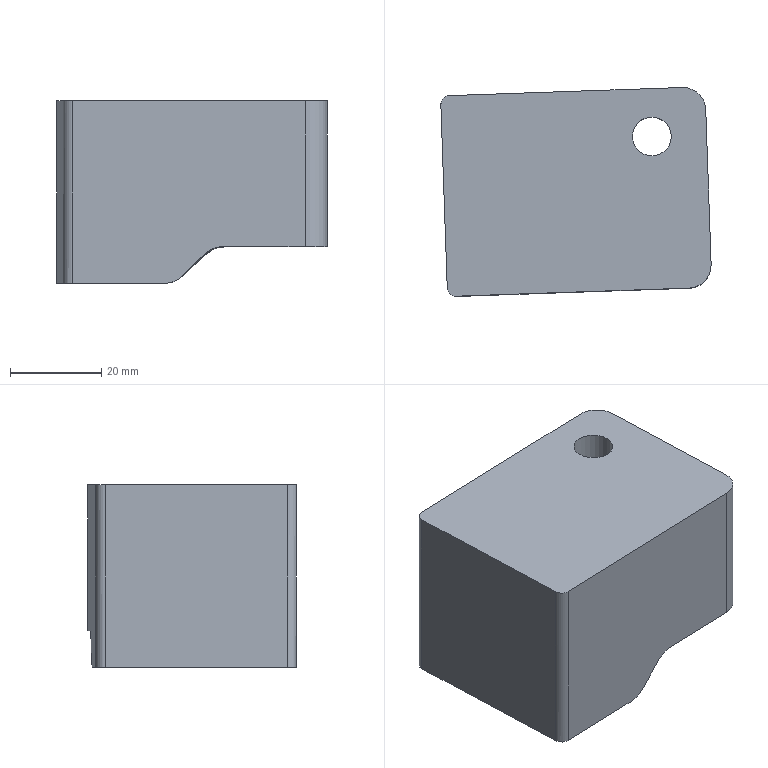Part | NX | features PS-16 2 | 1 solid | 16 faces | box 59.26 x 45.757 x 40 mm | volume 88557 mm3 | plane 8 | cylinder 6 | spline 2 | commonest cylinder face diameters 4 x2 10 x2 8.506 x1 14.5 x1
STEP:
#1=CARTESIAN_POINT('',(2975.173,-776.36,868.716));
#2=VERTEX_POINT('',#1);
#3=CARTESIAN_POINT('',(2958.185,-776.954,868.716));
#4=VERTEX_POINT('',#3);
#5=CARTESIAN_POINT('',(2937.196,-777.686,868.716));
#6=DIRECTION('',(-0.9994,-0.0349,0.));
#7=VECTOR('',#6,1000.);
#8=LINE('',#5,#7);
#9=EDGE_CURVE('',#2,#4,#8,.T.);
#10=ORIENTED_EDGE('',*,*,#9,.F.);
#11=CARTESIAN_POINT('',(2980.345,-781.183,868.716));
#12=VERTEX_POINT('',#11);
#13=CARTESIAN_POINT('',(2975.348,-781.357,868.716));
#14=DIRECTION('',(0.,0.,1.));
#15=DIRECTION('',(-1.,0.,0.));
#16=AXIS2_PLACEMENT_3D('',#13,#14,#15);
#17=CIRCLE('',#16,5.);
#18=EDGE_CURVE('',#12,#2,#17,.T.);
#19=ORIENTED_EDGE('',*,*,#18,.F.);
#20=CARTESIAN_POINT('',(2981.531,-815.162,868.716));
#21=VERTEX_POINT('',#20);
#22=CARTESIAN_POINT('',(2981.283,-808.048,868.716));
#23=DIRECTION('',(-0.0349,0.9994,0.));
#24=VECTOR('',#23,1000.);
#25=LINE('',#22,#24);
#26=EDGE_CURVE('',#21,#12,#25,.T.);
#27=ORIENTED_EDGE('',*,*,#26,.F.);
#28=CARTESIAN_POINT('',(2976.709,-820.334,868.716));
#29=VERTEX_POINT('',#28);
#30=CARTESIAN_POINT('',(2976.534,-815.337,868.716));
#31=DIRECTION('',(0.,0.,1.));
#32=DIRECTION('',(-1.,0.,0.));
#33=AXIS2_PLACEMENT_3D('',#30,#31,#32);
#34=CIRCLE('',#33,5.);
#35=EDGE_CURVE('',#29,#21,#34,.T.);
#36=ORIENTED_EDGE('',*,*,#35,.F.);
#37=CARTESIAN_POINT('',(2959.023,-820.951,868.716));
#38=VERTEX_POINT('',#37);
#39=CARTESIAN_POINT('',(2967.654,-820.65,868.716));
#40=DIRECTION('',(0.9994,0.0349,0.));
#41=VECTOR('',#40,1000.);
#42=LINE('',#39,#41);
#43=EDGE_CURVE('',#38,#29,#42,.T.);
#44=ORIENTED_EDGE('',*,*,#43,.F.);
#45=CARTESIAN_POINT('',(2958.185,-796.966,868.716));
#46=VERTEX_POINT('',#45);
#47=CARTESIAN_POINT('',(2958.011,-791.963,868.716));
#48=DIRECTION('',(-0.0349,0.9994,0.));
#49=VECTOR('',#48,1000.);
#50=LINE('',#47,#49);
#51=EDGE_CURVE('',#46,#38,#50,.F.);
#52=ORIENTED_EDGE('',*,*,#51,.F.);
#53=CARTESIAN_POINT('',(2958.185,-776.954,868.716));
#54=CARTESIAN_POINT('',(2958.185,-777.787,868.716));
#55=CARTESIAN_POINT('',(2958.185,-779.456,868.716));
#56=CARTESIAN_POINT('',(2958.185,-781.955,868.716));
#57=CARTESIAN_POINT('',(2958.185,-784.047,868.716));
#58=CARTESIAN_POINT('',(2958.185,-785.492,868.716));
#59=CARTESIAN_POINT('',(2958.185,-786.349,868.716));
#60=CARTESIAN_POINT('',(2958.185,-786.904,868.716));
#61=CARTESIAN_POINT('',(2958.185,-787.793,868.716));
#62=CARTESIAN_POINT('',(2958.185,-788.774,868.716));
#63=CARTESIAN_POINT('',(2958.185,-789.914,868.716));
#64=CARTESIAN_POINT('',(2958.185,-791.068,868.716));
#65=CARTESIAN_POINT('',(2958.185,-791.963,868.716));
#66=CARTESIAN_POINT('',(2958.185,-792.857,868.716));
#67=CARTESIAN_POINT('',(2958.185,-794.4,868.716));
#68=CARTESIAN_POINT('',(2958.185,-795.854,868.716));
#69=CARTESIAN_POINT('',(2958.185,-796.966,868.716));
#70=B_SPLINE_CURVE_WITH_KNOTS('',3,(#53,#54,#55,#56,#57,#58,#59,#60,#61,#62,#63,#64,#65,#66,#67,#68,#69),.UNSPECIFIED.,.F.,.F.,(4,1,1,1,1,1,1,1,1,1,1,1,1,1,4),(0.,0.125,0.25,0.375,0.4375,0.4688,0.5,0.5312,0.5625,0.625,0.6875,0.75,0.8125,0.875,1.),.UNSPECIFIED.);
#71=EDGE_CURVE('',#46,#4,#70,.F.);
#72=ORIENTED_EDGE('',*,*,#71,.T.);
#73=EDGE_LOOP('',(#10,#19,#27,#36,#44,#52,#72));
#74=FACE_BOUND('',#73,.T.);
#75=CARTESIAN_POINT('',(2975.794,-787.098,868.716));
#76=VERTEX_POINT('',#75);
#77=CARTESIAN_POINT('',(2968.544,-787.098,868.716));
#78=DIRECTION('',(0.,0.,-1.));
#79=DIRECTION('',(1.,0.,0.));
#80=AXIS2_PLACEMENT_3D('',#77,#78,#79);
#81=CIRCLE('',#80,7.25);
#82=EDGE_CURVE('',#76,#76,#81,.T.);
#83=ORIENTED_EDGE('',*,*,#82,.F.);
#84=EDGE_LOOP('',(#83));
#85=FACE_BOUND('',#84,.T.);
#86=CARTESIAN_POINT('',(2967.231,-808.539,868.716));
#87=DIRECTION('',(0.,0.,-1.));
#88=DIRECTION('',(0.0349,-0.9994,0.));
#89=AXIS2_PLACEMENT_3D('',#86,#87,#88);
#90=PLANE('',#89);
#91=ADVANCED_FACE('',(#74,#85),#90,.T.);
#92=CARTESIAN_POINT('',(2923.671,-820.184,900.716));
#93=VERTEX_POINT('',#92);
#94=CARTESIAN_POINT('',(2922.275,-780.209,900.716));
#95=VERTEX_POINT('',#94);
#96=CARTESIAN_POINT('',(2924.945,-856.656,900.716));
#97=DIRECTION('',(-0.0349,0.9994,0.));
#98=VECTOR('',#97,1000.);
#99=LINE('',#96,#98);
#100=EDGE_CURVE('',#93,#95,#99,.T.);
#101=ORIENTED_EDGE('',*,*,#100,.T.);
#102=CARTESIAN_POINT('',(2922.275,-780.209,860.716));
#103=VERTEX_POINT('',#102);
#104=CARTESIAN_POINT('',(2922.275,-780.209,862.716));
#105=DIRECTION('',(0.,0.,-1.));
#106=VECTOR('',#105,1000.);
#107=LINE('',#104,#106);
#108=EDGE_CURVE('',#103,#95,#107,.F.);
#109=ORIENTED_EDGE('',*,*,#108,.F.);
#110=CARTESIAN_POINT('',(2923.671,-820.184,860.716));
#111=VERTEX_POINT('',#110);
#112=CARTESIAN_POINT('',(2923.671,-820.184,860.716));
#113=CARTESIAN_POINT('',(2923.206,-806.859,860.716));
#114=CARTESIAN_POINT('',(2922.741,-793.534,860.716));
#115=CARTESIAN_POINT('',(2922.275,-780.209,860.716));
#116=B_SPLINE_CURVE_WITH_KNOTS('',3,(#112,#113,#114,#115),.UNSPECIFIED.,.F.,.F.,(4,4),(0.,0.04),.UNSPECIFIED.);
#117=EDGE_CURVE('',#111,#103,#116,.T.);
#118=ORIENTED_EDGE('',*,*,#117,.F.);
#119=CARTESIAN_POINT('',(2923.671,-820.184,862.716));
#120=DIRECTION('',(0.,0.,-1.));
#121=VECTOR('',#120,1000.);
#122=LINE('',#119,#121);
#123=EDGE_CURVE('',#93,#111,#122,.T.);
#124=ORIENTED_EDGE('',*,*,#123,.F.);
#125=EDGE_LOOP('',(#101,#109,#118,#124));
#126=FACE_BOUND('',#125,.T.);
#127=CARTESIAN_POINT('',(2923.132,-804.735,862.716));
#128=DIRECTION('',(0.9994,0.0349,0.));
#129=DIRECTION('',(0.0349,-0.9994,0.));
#130=AXIS2_PLACEMENT_3D('',#127,#128,#129);
#131=PLANE('',#130);
#132=ADVANCED_FACE('',(#126),#131,.F.);
#133=CARTESIAN_POINT('',(2981.531,-815.162,900.716));
#134=VERTEX_POINT('',#133);
#135=CARTESIAN_POINT('',(2981.531,-815.162,862.716));
#136=DIRECTION('',(0.,0.,1.));
#137=VECTOR('',#136,1000.);
#138=LINE('',#135,#137);
#139=EDGE_CURVE('',#21,#134,#138,.T.);
#140=ORIENTED_EDGE('',*,*,#139,.F.);
#141=ORIENTED_EDGE('',*,*,#26,.T.);
#142=CARTESIAN_POINT('',(2980.345,-781.183,900.716));
#143=VERTEX_POINT('',#142);
#144=CARTESIAN_POINT('',(2980.345,-781.183,935.716));
#145=DIRECTION('',(0.,0.,1.));
#146=VECTOR('',#145,1000.);
#147=LINE('',#144,#146);
#148=EDGE_CURVE('',#143,#12,#147,.F.);
#149=ORIENTED_EDGE('',*,*,#148,.F.);
#150=CARTESIAN_POINT('',(2982.909,-854.632,900.716));
#151=DIRECTION('',(-0.0349,0.9994,0.));
#152=VECTOR('',#151,1000.);
#153=LINE('',#150,#152);
#154=EDGE_CURVE('',#134,#143,#153,.T.);
#155=ORIENTED_EDGE('',*,*,#154,.F.);
#156=EDGE_LOOP('',(#140,#141,#149,#155));
#157=FACE_BOUND('',#156,.T.);
#158=CARTESIAN_POINT('',(2981.096,-802.711,862.716));
#159=DIRECTION('',(0.9994,0.0349,0.));
#160=DIRECTION('',(0.0349,-0.9994,0.));
#161=AXIS2_PLACEMENT_3D('',#158,#159,#160);
#162=PLANE('',#161);
#163=ADVANCED_FACE('',(#157),#162,.T.);
#164=CARTESIAN_POINT('',(2975.173,-776.36,900.716));
#165=VERTEX_POINT('',#164);
#166=CARTESIAN_POINT('',(2924.204,-778.14,900.716));
#167=VERTEX_POINT('',#166);
#168=CARTESIAN_POINT('',(2937.196,-777.686,900.716));
#169=DIRECTION('',(-0.9994,-0.0349,0.));
#170=VECTOR('',#169,1000.);
#171=LINE('',#168,#170);
#172=EDGE_CURVE('',#165,#167,#171,.T.);
#173=ORIENTED_EDGE('',*,*,#172,.F.);
#174=CARTESIAN_POINT('',(2975.173,-776.36,935.716));
#175=DIRECTION('',(0.,0.,1.));
#176=VECTOR('',#175,1000.);
#177=LINE('',#174,#176);
#178=EDGE_CURVE('',#2,#165,#177,.T.);
#179=ORIENTED_EDGE('',*,*,#178,.F.);
#180=ORIENTED_EDGE('',*,*,#9,.T.);
#181=CARTESIAN_POINT('',(2946.238,-777.371,860.716));
#182=VERTEX_POINT('',#181);
#183=CARTESIAN_POINT('',(2946.238,-777.371,860.716));
#184=CARTESIAN_POINT('',(2946.843,-777.35,860.716));
#185=CARTESIAN_POINT('',(2948.076,-777.307,860.995));
#186=CARTESIAN_POINT('',(2950.148,-777.234,862.36));
#187=CARTESIAN_POINT('',(2952.239,-777.161,864.66));
#188=CARTESIAN_POINT('',(2954.666,-777.076,867.458));
#189=CARTESIAN_POINT('',(2956.946,-776.997,868.716));
#190=CARTESIAN_POINT('',(2958.185,-776.954,868.716));
#191=B_SPLINE_CURVE_WITH_KNOTS('',3,(#183,#184,#185,#186,#187,#188,#189,#190),.UNSPECIFIED.,.F.,.F.,(4,1,1,1,1,4),(0.008073,0.009904,0.01173,0.0154,0.01906,0.02272),.UNSPECIFIED.);
#192=EDGE_CURVE('',#4,#182,#191,.F.);
#193=ORIENTED_EDGE('',*,*,#192,.T.);
#194=CARTESIAN_POINT('',(2924.204,-778.14,860.716));
#195=VERTEX_POINT('',#194);
#196=CARTESIAN_POINT('',(2924.204,-778.14,860.716));
#197=CARTESIAN_POINT('',(2931.549,-777.884,860.716));
#198=CARTESIAN_POINT('',(2938.894,-777.627,860.716));
#199=CARTESIAN_POINT('',(2946.238,-777.371,860.716));
#200=B_SPLINE_CURVE_WITH_KNOTS('',3,(#196,#197,#198,#199),.UNSPECIFIED.,.F.,.F.,(4,4),(0.,0.02205),.UNSPECIFIED.);
#201=EDGE_CURVE('',#195,#182,#200,.T.);
#202=ORIENTED_EDGE('',*,*,#201,.F.);
#203=CARTESIAN_POINT('',(2924.204,-778.14,935.716));
#204=DIRECTION('',(0.,0.,-1.));
#205=VECTOR('',#204,1000.);
#206=LINE('',#203,#205);
#207=EDGE_CURVE('',#167,#195,#206,.T.);
#208=ORIENTED_EDGE('',*,*,#207,.F.);
#209=EDGE_LOOP('',(#173,#179,#180,#193,#202,#208));
#210=FACE_BOUND('',#209,.T.);
#211=CARTESIAN_POINT('',(2937.196,-777.686,935.716));
#212=DIRECTION('',(0.0349,-0.9994,0.));
#213=DIRECTION('',(-0.9994,-0.0349,0.));
#214=AXIS2_PLACEMENT_3D('',#211,#212,#213);
#215=PLANE('',#214);
#216=ADVANCED_FACE('',(#210),#215,.F.);
#217=ORIENTED_EDGE('',*,*,#148,.T.);
#218=ORIENTED_EDGE('',*,*,#18,.T.);
#219=ORIENTED_EDGE('',*,*,#178,.T.);
#220=CARTESIAN_POINT('',(2975.348,-781.357,900.716));
#221=DIRECTION('',(0.,0.,1.));
#222=DIRECTION('',(1.,0.,0.));
#223=AXIS2_PLACEMENT_3D('',#220,#221,#222);
#224=CIRCLE('',#223,5.);
#225=EDGE_CURVE('',#143,#165,#224,.T.);
#226=ORIENTED_EDGE('',*,*,#225,.F.);
#227=EDGE_LOOP('',(#217,#218,#219,#226));
#228=FACE_BOUND('',#227,.T.);
#229=CARTESIAN_POINT('',(2975.348,-781.357,935.716));
#230=DIRECTION('',(0.,0.,-1.));
#231=DIRECTION('',(-1.,0.,0.));
#232=AXIS2_PLACEMENT_3D('',#229,#230,#231);
#233=CYLINDRICAL_SURFACE('',#232,5.);
#234=ADVANCED_FACE('',(#228),#233,.T.);
#235=ORIENTED_EDGE('',*,*,#207,.T.);
#236=CARTESIAN_POINT('',(2924.204,-778.14,860.716));
#237=CARTESIAN_POINT('',(2923.676,-778.158,860.716));
#238=CARTESIAN_POINT('',(2922.657,-778.629,860.716));
#239=CARTESIAN_POINT('',(2922.257,-779.681,860.716));
#240=CARTESIAN_POINT('',(2922.275,-780.209,860.716));
#241=B_SPLINE_CURVE_WITH_KNOTS('',3,(#236,#237,#238,#239,#240),.UNSPECIFIED.,.F.,.F.,(4,1,4),(0.,0.001562,0.003124),.UNSPECIFIED.);
#242=EDGE_CURVE('',#195,#103,#241,.T.);
#243=ORIENTED_EDGE('',*,*,#242,.T.);
#244=ORIENTED_EDGE('',*,*,#108,.T.);
#245=CARTESIAN_POINT('',(2924.274,-780.139,900.716));
#246=DIRECTION('',(0.,0.,1.));
#247=DIRECTION('',(1.,0.,0.));
#248=AXIS2_PLACEMENT_3D('',#245,#246,#247);
#249=CIRCLE('',#248,2.);
#250=EDGE_CURVE('',#167,#95,#249,.T.);
#251=ORIENTED_EDGE('',*,*,#250,.F.);
#252=EDGE_LOOP('',(#235,#243,#244,#251));
#253=FACE_BOUND('',#252,.T.);
#254=CARTESIAN_POINT('',(2924.274,-780.139,935.716));
#255=DIRECTION('',(0.,0.,-1.));
#256=DIRECTION('',(-1.,0.,0.));
#257=AXIS2_PLACEMENT_3D('',#254,#255,#256);
#258=CYLINDRICAL_SURFACE('',#257,2.);
#259=ADVANCED_FACE('',(#253),#258,.T.);
#260=CARTESIAN_POINT('',(2925.74,-822.113,860.716));
#261=VERTEX_POINT('',#260);
#262=CARTESIAN_POINT('',(2925.74,-822.113,900.716));
#263=VERTEX_POINT('',#262);
#264=CARTESIAN_POINT('',(2925.74,-822.113,862.716));
#265=DIRECTION('',(0.,0.,-1.));
#266=VECTOR('',#265,1000.);
#267=LINE('',#264,#266);
#268=EDGE_CURVE('',#261,#263,#267,.F.);
#269=ORIENTED_EDGE('',*,*,#268,.T.);
#270=CARTESIAN_POINT('',(2925.67,-820.114,900.716));
#271=DIRECTION('',(0.,0.,1.));
#272=DIRECTION('',(1.,0.,0.));
#273=AXIS2_PLACEMENT_3D('',#270,#271,#272);
#274=CIRCLE('',#273,2.);
#275=EDGE_CURVE('',#93,#263,#274,.T.);
#276=ORIENTED_EDGE('',*,*,#275,.F.);
#277=ORIENTED_EDGE('',*,*,#123,.T.);
#278=CARTESIAN_POINT('',(2925.74,-822.113,860.716));
#279=CARTESIAN_POINT('',(2925.212,-822.132,860.716));
#280=CARTESIAN_POINT('',(2924.162,-821.733,860.716));
#281=CARTESIAN_POINT('',(2923.69,-820.712,860.716));
#282=CARTESIAN_POINT('',(2923.671,-820.184,860.716));
#283=B_SPLINE_CURVE_WITH_KNOTS('',3,(#278,#279,#280,#281,#282),.UNSPECIFIED.,.F.,.F.,(4,1,4),(0.,0.001562,0.003124),.UNSPECIFIED.);
#284=EDGE_CURVE('',#261,#111,#283,.T.);
#285=ORIENTED_EDGE('',*,*,#284,.F.);
#286=EDGE_LOOP('',(#269,#276,#277,#285));
#287=FACE_BOUND('',#286,.T.);
#288=CARTESIAN_POINT('',(2925.67,-820.114,862.716));
#289=DIRECTION('',(0.,0.,1.));
#290=DIRECTION('',(1.,0.,0.));
#291=AXIS2_PLACEMENT_3D('',#288,#289,#290);
#292=CYLINDRICAL_SURFACE('',#291,2.);
#293=ADVANCED_FACE('',(#287),#292,.T.);
#294=CARTESIAN_POINT('',(2946.238,-821.397,860.716));
#295=VERTEX_POINT('',#294);
#296=CARTESIAN_POINT('',(2925.74,-822.113,860.716));
#297=CARTESIAN_POINT('',(2932.573,-821.875,860.716));
#298=CARTESIAN_POINT('',(2939.405,-821.636,860.716));
#299=CARTESIAN_POINT('',(2946.238,-821.397,860.716));
#300=B_SPLINE_CURVE_WITH_KNOTS('',3,(#296,#297,#298,#299),.UNSPECIFIED.,.F.,.F.,(4,4),(0.,0.02051),.UNSPECIFIED.);
#301=EDGE_CURVE('',#261,#295,#300,.T.);
#302=ORIENTED_EDGE('',*,*,#301,.T.);
#303=CARTESIAN_POINT('',(2959.023,-820.951,868.669));
#304=VERTEX_POINT('',#303);
#305=CARTESIAN_POINT('',(2959.023,-820.951,868.669));
#306=CARTESIAN_POINT('',(2958.366,-820.974,868.724));
#307=CARTESIAN_POINT('',(2957.025,-821.021,868.727));
#308=CARTESIAN_POINT('',(2955.255,-821.083,867.728));
#309=CARTESIAN_POINT('',(2953.812,-821.133,866.413));
#310=CARTESIAN_POINT('',(2952.048,-821.195,864.489));
#311=CARTESIAN_POINT('',(2949.934,-821.268,862.017));
#312=CARTESIAN_POINT('',(2947.53,-821.352,860.716));
#313=CARTESIAN_POINT('',(2946.238,-821.397,860.716));
#314=B_SPLINE_CURVE_WITH_KNOTS('',3,(#305,#306,#307,#308,#309,#310,#311,#312,#313),.UNSPECIFIED.,.F.,.F.,(4,1,1,1,1,1,4),(0.04332,0.0453,0.04728,0.04926,0.05123,0.05519,0.05914),.UNSPECIFIED.);
#315=EDGE_CURVE('',#304,#295,#314,.T.);
#316=ORIENTED_EDGE('',*,*,#315,.F.);
#317=CARTESIAN_POINT('',(2959.023,-820.951,927.716));
#318=DIRECTION('',(0.,0.,-1.));
#319=VECTOR('',#318,1000.);
#320=LINE('',#317,#319);
#321=EDGE_CURVE('',#304,#38,#320,.F.);
#322=ORIENTED_EDGE('',*,*,#321,.T.);
#323=ORIENTED_EDGE('',*,*,#43,.T.);
#324=CARTESIAN_POINT('',(2976.709,-820.334,900.716));
#325=VERTEX_POINT('',#324);
#326=CARTESIAN_POINT('',(2976.709,-820.334,935.716));
#327=DIRECTION('',(0.,0.,1.));
#328=VECTOR('',#327,1000.);
#329=LINE('',#326,#328);
#330=EDGE_CURVE('',#325,#29,#329,.F.);
#331=ORIENTED_EDGE('',*,*,#330,.F.);
#332=CARTESIAN_POINT('',(2881.726,-823.65,900.716));
#333=DIRECTION('',(0.9994,0.0349,0.));
#334=VECTOR('',#333,1000.);
#335=LINE('',#332,#334);
#336=EDGE_CURVE('',#263,#325,#335,.T.);
#337=ORIENTED_EDGE('',*,*,#336,.F.);
#338=ORIENTED_EDGE('',*,*,#268,.F.);
#339=EDGE_LOOP('',(#302,#316,#322,#323,#331,#337,#338));
#340=FACE_BOUND('',#339,.T.);
#341=CARTESIAN_POINT('',(2938.732,-821.66,935.716));
#342=DIRECTION('',(0.0349,-0.9994,0.));
#343=DIRECTION('',(-0.9994,-0.0349,0.));
#344=AXIS2_PLACEMENT_3D('',#341,#342,#343);
#345=PLANE('',#344);
#346=ADVANCED_FACE('',(#340),#345,.T.);
#347=ORIENTED_EDGE('',*,*,#330,.T.);
#348=ORIENTED_EDGE('',*,*,#35,.T.);
#349=ORIENTED_EDGE('',*,*,#139,.T.);
#350=CARTESIAN_POINT('',(2976.534,-815.337,900.716));
#351=DIRECTION('',(0.,0.,1.));
#352=DIRECTION('',(1.,0.,0.));
#353=AXIS2_PLACEMENT_3D('',#350,#351,#352);
#354=CIRCLE('',#353,5.);
#355=EDGE_CURVE('',#134,#325,#354,.F.);
#356=ORIENTED_EDGE('',*,*,#355,.T.);
#357=EDGE_LOOP('',(#347,#348,#349,#356));
#358=FACE_BOUND('',#357,.T.);
#359=CARTESIAN_POINT('',(2976.534,-815.337,862.716));
#360=DIRECTION('',(0.,0.,1.));
#361=DIRECTION('',(1.,0.,0.));
#362=AXIS2_PLACEMENT_3D('',#359,#360,#361);
#363=CYLINDRICAL_SURFACE('',#362,5.);
#364=ADVANCED_FACE('',(#358),#363,.T.);
#365=ORIENTED_EDGE('',*,*,#51,.T.);
#366=ORIENTED_EDGE('',*,*,#321,.F.);
#367=CARTESIAN_POINT('',(2959.023,-820.951,868.669));
#368=CARTESIAN_POINT('',(2958.744,-812.956,868.692));
#369=CARTESIAN_POINT('',(2958.464,-804.961,868.716));
#370=CARTESIAN_POINT('',(2958.185,-796.966,868.716));
#371=B_SPLINE_CURVE_WITH_KNOTS('',3,(#367,#368,#369,#370),.UNSPECIFIED.,.F.,.F.,(4,4),(0.008665,0.03266),.UNSPECIFIED.);
#372=EDGE_CURVE('',#304,#46,#371,.T.);
#373=ORIENTED_EDGE('',*,*,#372,.T.);
#374=EDGE_LOOP('',(#365,#366,#373));
#375=FACE_BOUND('',#374,.T.);
#376=CARTESIAN_POINT('',(2958.011,-791.963,927.716));
#377=DIRECTION('',(-0.9994,-0.0349,0.));
#378=DIRECTION('',(-0.0349,0.9994,0.));
#379=AXIS2_PLACEMENT_3D('',#376,#377,#378);
#380=PLANE('',#379);
#381=ADVANCED_FACE('',(#375),#380,.F.);
#382=ORIENTED_EDGE('',*,*,#372,.F.);
#383=ORIENTED_EDGE('',*,*,#315,.T.);
#384=CARTESIAN_POINT('',(2946.238,-809.389,860.716));
#385=DIRECTION('',(0.,1.,0.));
#386=VECTOR('',#385,1000.);
#387=LINE('',#384,#386);
#388=EDGE_CURVE('',#295,#182,#387,.T.);
#389=ORIENTED_EDGE('',*,*,#388,.T.);
#390=ORIENTED_EDGE('',*,*,#192,.F.);
#391=ORIENTED_EDGE('',*,*,#71,.F.);
#392=EDGE_LOOP('',(#382,#383,#389,#390,#391));
#393=FACE_BOUND('',#392,.T.);
#394=CARTESIAN_POINT('',(2959.119,-821.664,868.66));
#395=CARTESIAN_POINT('',(2959.119,-776.687,868.66));
#396=CARTESIAN_POINT('',(2958.445,-821.664,868.718));
#397=CARTESIAN_POINT('',(2958.445,-776.687,868.718));
#398=CARTESIAN_POINT('',(2957.101,-821.664,868.749));
#399=CARTESIAN_POINT('',(2957.101,-776.687,868.749));
#400=CARTESIAN_POINT('',(2955.329,-821.664,867.784));
#401=CARTESIAN_POINT('',(2955.329,-776.687,867.784));
#402=CARTESIAN_POINT('',(2953.865,-821.664,866.468));
#403=CARTESIAN_POINT('',(2953.865,-776.687,866.468));
#404=CARTESIAN_POINT('',(2952.091,-821.664,864.539));
#405=CARTESIAN_POINT('',(2952.091,-776.687,864.539));
#406=CARTESIAN_POINT('',(2949.974,-821.664,862.058));
#407=CARTESIAN_POINT('',(2949.974,-776.687,862.058));
#408=CARTESIAN_POINT('',(2947.562,-821.664,860.716));
#409=CARTESIAN_POINT('',(2947.562,-776.687,860.716));
#410=CARTESIAN_POINT('',(2946.238,-821.664,860.716));
#411=CARTESIAN_POINT('',(2946.238,-776.687,860.716));
#412=B_SPLINE_SURFACE_WITH_KNOTS('',3,1,((#394,#395),(#396,#397),(#398,#399),(#400,#401),(#402,#403),(#404,#405),(#406,#407),(#408,#409),(#410,#411)),.SURF_OF_LINEAR_EXTRUSION.,.F.,.F.,.F.,(4,1,1,1,1,1,4),(2,2),(-0.06154,0.07115,0.2038,0.3365,0.4692,0.7346,1.),(0.,1.),.UNSPECIFIED.);
#413=ADVANCED_FACE('',(#393),#412,.T.);
#414=ORIENTED_EDGE('',*,*,#284,.T.);
#415=ORIENTED_EDGE('',*,*,#117,.T.);
#416=ORIENTED_EDGE('',*,*,#242,.F.);
#417=ORIENTED_EDGE('',*,*,#201,.T.);
#418=ORIENTED_EDGE('',*,*,#388,.F.);
#419=ORIENTED_EDGE('',*,*,#301,.F.);
#420=EDGE_LOOP('',(#414,#415,#416,#417,#418,#419));
#421=FACE_BOUND('',#420,.T.);
#422=CARTESIAN_POINT('',(2916.687,-770.111,860.716));
#423=CARTESIAN_POINT('',(2914.756,-825.438,860.716));
#424=CARTESIAN_POINT('',(2912.824,-880.765,860.716));
#425=CARTESIAN_POINT('',(2910.892,-936.091,860.716));
#426=CARTESIAN_POINT('',(3023.952,-773.857,860.716));
#427=CARTESIAN_POINT('',(3022.02,-829.183,860.716));
#428=CARTESIAN_POINT('',(3020.088,-884.51,860.716));
#429=CARTESIAN_POINT('',(3018.157,-939.837,860.716));
#430=B_SPLINE_SURFACE_WITH_KNOTS('',1,3,((#422,#423,#424,#425),(#426,#427,#428,#429)),.PLANE_SURF.,.F.,.F.,.F.,(2,2),(4,4),(-20.466,1.),(-2.61,1.),.PIECEWISE_BEZIER_KNOTS.);
#431=ADVANCED_FACE('',(#421),#430,.T.);
#432=CARTESIAN_POINT('',(2972.797,-787.098,900.716));
#433=VERTEX_POINT('',#432);
#434=CARTESIAN_POINT('',(2968.544,-787.098,900.716));
#435=DIRECTION('',(0.,0.,1.));
#436=DIRECTION('',(1.,0.,0.));
#437=AXIS2_PLACEMENT_3D('',#434,#435,#436);
#438=CIRCLE('',#437,4.253);
#439=EDGE_CURVE('',#433,#433,#438,.F.);
#440=ORIENTED_EDGE('',*,*,#439,.T.);
#441=EDGE_LOOP('',(#440));
#442=FACE_BOUND('',#441,.T.);
#443=ORIENTED_EDGE('',*,*,#250,.T.);
#444=ORIENTED_EDGE('',*,*,#100,.F.);
#445=ORIENTED_EDGE('',*,*,#275,.T.);
#446=ORIENTED_EDGE('',*,*,#336,.T.);
#447=ORIENTED_EDGE('',*,*,#355,.F.);
#448=ORIENTED_EDGE('',*,*,#154,.T.);
#449=ORIENTED_EDGE('',*,*,#225,.T.);
#450=ORIENTED_EDGE('',*,*,#172,.T.);
#451=EDGE_LOOP('',(#443,#444,#445,#446,#447,#448,#449,#450));
#452=FACE_BOUND('',#451,.T.);
#453=CARTESIAN_POINT('',(2882.93,-858.123,900.716));
#454=DIRECTION('',(0.,0.,1.));
#455=DIRECTION('',(1.,0.,0.));
#456=AXIS2_PLACEMENT_3D('',#453,#454,#455);
#457=PLANE('',#456);
#458=ADVANCED_FACE('',(#442,#452),#457,.T.);
#459=ORIENTED_EDGE('',*,*,#439,.F.);
#460=EDGE_LOOP('',(#459));
#461=FACE_BOUND('',#460,.T.);
#462=CARTESIAN_POINT('',(2972.797,-787.098,879.716));
#463=VERTEX_POINT('',#462);
#464=CARTESIAN_POINT('',(2968.544,-787.098,879.716));
#465=DIRECTION('',(0.,0.,-1.));
#466=DIRECTION('',(1.,0.,0.));
#467=AXIS2_PLACEMENT_3D('',#464,#465,#466);
#468=CIRCLE('',#467,4.253);
#469=EDGE_CURVE('',#463,#463,#468,.T.);
#470=ORIENTED_EDGE('',*,*,#469,.T.);
#471=EDGE_LOOP('',(#470));
#472=FACE_BOUND('',#471,.T.);
#473=CARTESIAN_POINT('',(2968.544,-787.098,868.716));
#474=DIRECTION('',(0.,0.,1.));
#475=DIRECTION('',(1.,0.,0.));
#476=AXIS2_PLACEMENT_3D('',#473,#474,#475);
#477=CYLINDRICAL_SURFACE('',#476,4.253);
#478=ADVANCED_FACE('',(#461,#472),#477,.F.);
#479=ORIENTED_EDGE('',*,*,#469,.F.);
#480=EDGE_LOOP('',(#479));
#481=FACE_BOUND('',#480,.T.);
#482=CARTESIAN_POINT('',(2975.794,-787.098,879.716));
#483=VERTEX_POINT('',#482);
#484=CARTESIAN_POINT('',(2968.544,-787.098,879.716));
#485=DIRECTION('',(0.,0.,1.));
#486=DIRECTION('',(1.,0.,0.));
#487=AXIS2_PLACEMENT_3D('',#484,#485,#486);
#488=CIRCLE('',#487,7.25);
#489=EDGE_CURVE('',#483,#483,#488,.F.);
#490=ORIENTED_EDGE('',*,*,#489,.T.);
#491=EDGE_LOOP('',(#490));
#492=FACE_BOUND('',#491,.T.);
#493=CARTESIAN_POINT('',(2968.544,-787.098,879.716));
#494=DIRECTION('',(0.,0.,1.));
#495=DIRECTION('',(1.,0.,0.));
#496=AXIS2_PLACEMENT_3D('',#493,#494,#495);
#497=PLANE('',#496);
#498=ADVANCED_FACE('',(#481,#492),#497,.F.);
#499=ORIENTED_EDGE('',*,*,#489,.F.);
#500=EDGE_LOOP('',(#499));
#501=FACE_BOUND('',#500,.T.);
#502=ORIENTED_EDGE('',*,*,#82,.T.);
#503=EDGE_LOOP('',(#502));
#504=FACE_BOUND('',#503,.T.);
#505=CARTESIAN_POINT('',(2968.544,-787.098,868.716));
#506=DIRECTION('',(0.,0.,1.));
#507=DIRECTION('',(1.,0.,0.));
#508=AXIS2_PLACEMENT_3D('',#505,#506,#507);
#509=CYLINDRICAL_SURFACE('',#508,7.25);
#510=ADVANCED_FACE('',(#501,#504),#509,.F.);
#511=CLOSED_SHELL('',(#91,#132,#163,#216,#234,#259,#293,#346,#364,#381,#413,#431,#458,#478,#498,#510));
#512=MANIFOLD_SOLID_BREP('',#511);
#513=(LENGTH_UNIT()NAMED_UNIT(*)SI_UNIT(.MILLI.,.METRE.));
#514=UNCERTAINTY_MEASURE_WITH_UNIT(LENGTH_MEASURE(0.0508),#513,'','');
#515=(NAMED_UNIT(*)PLANE_ANGLE_UNIT()SI_UNIT($,.RADIAN.));
#516=(NAMED_UNIT(*)SI_UNIT($,.STERADIAN.)SOLID_ANGLE_UNIT());
#517=(GEOMETRIC_REPRESENTATION_CONTEXT(3)GLOBAL_UNCERTAINTY_ASSIGNED_CONTEXT((#514))GLOBAL_UNIT_ASSIGNED_CONTEXT((#513,#515,#516))REPRESENTATION_CONTEXT('',''));
#518=ADVANCED_BREP_SHAPE_REPRESENTATION('',(#512),#517);